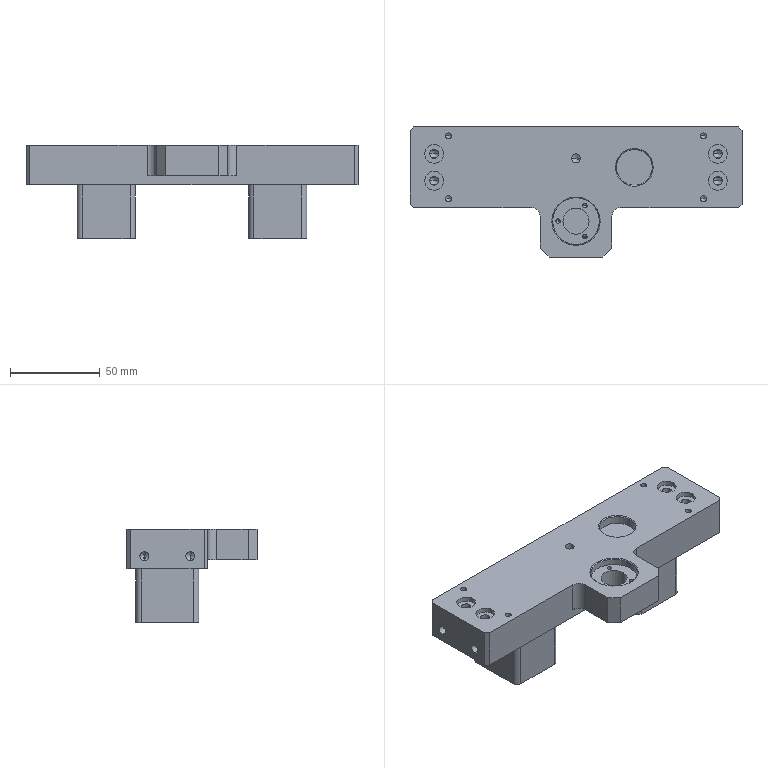NC program | NX | posted with a generic post | part box 185 x 72.5 x 52 mm
Whole program:
N10 G17 G21 G94 G90
(ZLEVEL_PROFILE_1 , TOOL : D10)
N12 T15 M6
N14 G54
N16 G17 G0 G90 X-108.145 Y0.067 S9500 M3
N18 G43 Z30. H15
N20 Z3.429
N22 G94 G1 Z2.429 F1000.
N24 X-107.651 Y0.199
N26 G2 X-106.685 Y-0.06 R1.
N28 G1 X-96.649 Y-10.096 F2500.
N30 X-96.62 Y-10.084
N32 G3 X-96.248 Y-10.498 R5.3
N34 G1 X-94.248 Y-12.498
N36 G3 X-90.5 Y-14.05 R5.3
N38 G1 X-25.3
N40 Y-30.19
N42 X-25.296 Y-30.622
N44 X-25.269 Y-30.673
N46 G3 X-23.748 Y-34.998 R5.3
N48 G1 X-18.748 Y-39.998
N50 G3 X-15. Y-41.55 R5.3
N52 G1 X15.
N54 G3 X18.748 Y-39.998 R5.3
N56 G1 X23.748 Y-34.998
N58 G3 X25.269 Y-30.673 R5.3
N60 G1 X25.296 Y-30.622
N62 Y-30.238
N64 X25.3 Y-30.19
N66 Y-14.05
N68 X90.5
N70 G3 X94.763 Y-11.9 R5.3
N72 G1 X94.829 Y-11.911
N74 X94.952 Y-11.788
N76 X94.979 Y-11.766
N78 X96.218 Y-10.527
N80 X106.852 Y0.107
N82 G2 X107.818 Y0.366 R1.
N84 G1 X108.268 Y0.246
N86 Z3.429
N88 G0 Z68.
N90 X-108.145 Y0.067
N92 Z2.857
N94 G1 Z1.857 F1000.
N96 X-107.651 Y0.199
N98 G2 X-106.685 Y-0.06 R1.
N100 G1 X-96.649 Y-10.096 F2500.
N102 X-96.62 Y-10.084
N104 G3 X-96.248 Y-10.498 R5.3
N106 G1 X-94.248 Y-12.498
N108 G3 X-90.5 Y-14.05 R5.3
N110 G1 X-25.3
N112 Y-30.19
N114 X-25.296 Y-30.622
N116 X-25.269 Y-30.673
N118 G3 X-23.748 Y-34.998 R5.3
N120 G1 X-18.748 Y-39.998
N122 G3 X-15. Y-41.55 R5.3
N124 G1 X15.
N126 G3 X18.748 Y-39.998 R5.3
N128 G1 X23.748 Y-34.998
N130 G3 X25.269 Y-30.673 R5.3
N132 G1 X25.296 Y-30.622
N134 Y-30.238
N136 X25.3 Y-30.19
N138 Y-14.05
N140 X90.5
N142 G3 X94.763 Y-11.9 R5.3
N144 G1 X94.829 Y-11.911
N146 X94.952 Y-11.788
N148 X94.979 Y-11.766
N150 X96.218 Y-10.527
N152 X106.852 Y0.107
N154 G2 X107.818 Y0.366 R1.
N156 G1 X108.268 Y0.246
N158 Z2.857
N160 G0 Z68.
N162 X-108.145 Y0.067
N164 Z2.286
N166 G1 Z1.286 F1000.
N168 X-107.651 Y0.199
N170 G2 X-106.685 Y-0.06 R1.
N172 G1 X-96.649 Y-10.096 F2500.
N174 X-96.62 Y-10.084
N176 G3 X-96.248 Y-10.498 R5.3
N178 G1 X-94.248 Y-12.498
N180 G3 X-90.5 Y-14.05 R5.3
N182 G1 X-25.3
N184 Y-30.19
N186 X-25.296 Y-30.622
N188 X-25.269 Y-30.673
N190 G3 X-23.748 Y-34.998 R5.3
N192 G1 X-18.748 Y-39.998
N194 G3 X-15. Y-41.55 R5.3
N196 G1 X15.
N198 G3 X18.748 Y-39.998 R5.3
N200 G1 X23.748 Y-34.998
N202 G3 X25.269 Y-30.673 R5.3
N204 G1 X25.296 Y-30.622
N206 Y-30.238
N208 X25.3 Y-30.19
N210 Y-14.05
N212 X90.5
N214 G3 X94.763 Y-11.9 R5.3
N216 G1 X94.829 Y-11.911
N218 X94.952 Y-11.788
N220 X94.979 Y-11.766
N222 X96.218 Y-10.527
N224 X106.852 Y0.107
N226 G2 X107.818 Y0.366 R1.
N228 G1 X108.268 Y0.246
N230 Z2.286
N232 G0 Z68.
N234 X-108.145 Y0.067
N236 Z1.714
N238 G1 Z0.714 F1000.
N240 X-107.651 Y0.199
N242 G2 X-106.685 Y-0.06 R1.
N244 G1 X-96.649 Y-10.096 F2500.
N246 X-96.62 Y-10.084
N248 G3 X-96.248 Y-10.498 R5.3
N250 G1 X-94.248 Y-12.498
N252 G3 X-90.5 Y-14.05 R5.3
N254 G1 X-25.3
N256 Y-30.19
N258 X-25.296 Y-30.622
N260 X-25.269 Y-30.673
N262 G3 X-23.748 Y-34.998 R5.3
N264 G1 X-18.748 Y-39.998
N266 G3 X-15. Y-41.55 R5.3
N268 G1 X15.
N270 G3 X18.748 Y-39.998 R5.3
N272 G1 X23.748 Y-34.998
N274 G3 X25.269 Y-30.673 R5.3
N276 G1 X25.296 Y-30.622
N278 Y-30.238
N280 X25.3 Y-30.19
N282 Y-14.05
N284 X90.5
N286 G3 X94.763 Y-11.9 R5.3
N288 G1 X94.829 Y-11.911
N290 X94.952 Y-11.788
N292 X94.979 Y-11.766
N294 X96.218 Y-10.527
N296 X106.852 Y0.107
N298 G2 X107.818 Y0.366 R1.
N300 G1 X108.268 Y0.246
N302 Z1.714
N304 G0 Z68.
N306 X-108.145 Y0.067
N308 Z1.143
N310 G1 Z0.143 F1000.
N312 X-107.651 Y0.199
N314 G2 X-106.685 Y-0.06 R1.
N316 G1 X-96.649 Y-10.096 F2500.
N318 X-96.62 Y-10.084
N320 G3 X-96.248 Y-10.498 R5.3
N322 G1 X-94.248 Y-12.498
N324 G3 X-90.5 Y-14.05 R5.3
N326 G1 X-25.3
N328 Y-30.19
N330 X-25.296 Y-30.622
N332 X-25.269 Y-30.673
N334 G3 X-23.748 Y-34.998 R5.3
N336 G1 X-18.748 Y-39.998
N338 G3 X-15. Y-41.55 R5.3
N340 G1 X15.
N342 G3 X18.748 Y-39.998 R5.3
N344 G1 X23.748 Y-34.998
N346 G3 X25.269 Y-30.673 R5.3
N348 G1 X25.296 Y-30.622
N350 Y-30.238
N352 X25.3 Y-30.19
N354 Y-14.05
N356 X90.5
N358 G3 X94.763 Y-11.9 R5.3
N360 G1 X94.829 Y-11.911
N362 X94.952 Y-11.788
N364 X94.979 Y-11.766
N366 X96.218 Y-10.527
N368 X106.852 Y0.107
N370 G2 X107.818 Y0.366 R1.
N372 G1 X108.268 Y0.246
N374 Z1.143
N376 G0 Z68.
N378 X-108.145 Y0.067
N380 Z0.571
N382 G1 Z-0.429 F1000.
N384 X-107.651 Y0.199
N386 G2 X-106.685 Y-0.06 R1.
N388 G1 X-96.649 Y-10.096 F2500.
N390 X-96.62 Y-10.084
N392 G3 X-96.248 Y-10.498 R5.3
N394 G1 X-94.248 Y-12.498
N396 G3 X-90.5 Y-14.05 R5.3
N398 G1 X-25.3
N400 Y-30.19
N402 X-25.296 Y-30.622
N404 X-25.269 Y-30.673
N406 G3 X-23.748 Y-34.998 R5.3
N408 G1 X-18.748 Y-39.998
N410 G3 X-15. Y-41.55 R5.3
N412 G1 X15.
N414 G3 X18.748 Y-39.998 R5.3
N416 G1 X23.748 Y-34.998
N418 G3 X25.269 Y-30.673 R5.3
N420 G1 X25.296 Y-30.622
N422 Y-30.238
N424 X25.3 Y-30.19
N426 Y-14.05
N428 X90.5
N430 G3 X94.763 Y-11.9 R5.3
N432 G1 X94.829 Y-11.911
N434 X94.952 Y-11.788
N436 X94.979 Y-11.766
N438 X96.218 Y-10.527
N440 X106.852 Y0.107
N442 G2 X107.818 Y0.366 R1.
N444 G1 X108.268 Y0.246
N446 Z0.571
N448 G0 Z68.
N450 X-108.145 Y0.067
N452 Z0.
N454 G1 Z-1. F1000.
N456 X-107.651 Y0.199
N458 G2 X-106.685 Y-0.06 R1.
N460 G1 X-96.649 Y-10.096 F2500.
N462 X-96.62 Y-10.084
N464 G3 X-96.248 Y-10.498 R5.3
N466 G1 X-94.248 Y-12.498
N468 G3 X-90.5 Y-14.05 R5.3
N470 G1 X-25.3
N472 Y-30.19
N474 X-25.296 Y-30.622
N476 X-25.269 Y-30.673
N478 G3 X-23.748 Y-34.998 R5.3
N480 G1 X-18.748 Y-39.998
N482 G3 X-15. Y-41.55 R5.3
N484 G1 X15.
N486 G3 X18.748 Y-39.998 R5.3
N488 G1 X23.748 Y-34.998
N490 G3 X25.269 Y-30.673 R5.3
N492 G1 X25.296 Y-30.622
N494 Y-30.238
N496 X25.3 Y-30.19
N498 Y-14.05
N500 X90.5
N502 G3 X94.763 Y-11.9 R5.3
N504 G1 X94.829 Y-11.911
N506 X94.952 Y-11.788
N508 X94.979 Y-11.766
N510 X96.218 Y-10.527
N512 X106.852 Y0.107
N514 G2 X107.818 Y0.366 R1.
N516 G1 X108.268 Y0.246
N518 Z0.
N520 G0 Z30.
N522 M5
(FLOOR_WALL_COPY_COPY , TOOL : D80)
N524 T19 M6
N526 G54
N528 G17 G0 G90 X-137.5 Y36.247 S6500 M3
N530 G43 Z30. H19
N532 Z5.
N534 G94 G1 Z2. F1500.
N536 X-132.5
N538 X132.5
N540 Y-4.25
N542 X-132.5
N544 X-137.5
N546 Z5.
N548 G0 Z30.
N550 Y36.247
N552 Z4.
N554 G1 Z1.
N556 X-132.5
N558 X132.5
N560 Y-4.25
N562 X-132.5
N564 X-137.5
N566 Z4.
N568 G0 Z30.
N570 Y36.247
N572 Z3.
N574 G1 Z0.
N576 X-132.5
N578 X132.5
N580 Y-4.25
N582 X-132.5
N584 X-137.5
N586 Z3.
N588 G0 Z30.
N590 M5
(DRILLING_COPY_1_COPY , TOOL : D6A45)
N592 T01 M6
N594 G54
N596 G17 G0 G90 X71. Y-3.75 S5000 M3
N598 G43 Z30. H1
N600 G94 G81 G98 Z-1. F350. R3.
N602 X79. Y6.25
N604 Y21.25
N606 X71. Y31.25
N608 X32.5 Y13.75
N610 X0. Y18.75
N612 X5. Y-7.59
N614 X0. Y-16.25
N616 X5. Y-24.91
N618 X-10. Y-16.25
N620 X-71. Y-3.75
N622 X-79. Y6.25
N624 Y21.25
N626 X-71. Y31.25
N628 G80
N630 G0 X-71. Y31.25 Z30.
N632 M5
(DRILLING_COPY_COPY_1 , TOOL : 3.3ZT)
N634 T03 M6
N636 G54
N638 G17 G0 G90 X-71. Y-3.75 S2000 M3
N640 G43 Z30. H3
N642 G94 G83 G98 Z-10.491 F180. Q2. R3.
N644 Y31.25
N646 X71.
N648 Y-3.75
N650 G80
N652 G0 X71. Y-3.75 Z30.
(DRILLING_COPY_COPY_1_COPY_1 , TOOL : 3.3ZT)
N654 X0. Y18.75
N656 G83 Z-8.491 F180. Q2. R3.
N658 G80
N660 G0 X0. Y18.75 Z30.
N662 M5
(DRILLING_COPY_COPY_1_COPY , TOOL : 2.5ZT)
N664 T02 M6
N666 G54
N668 G17 G0 G90 X-10. Y-16.25 S2006 M3
N670 G43 Z30. H2
N672 G94 G83 G98 Z-12.251 F120. Q2. R3.
N674 X5. Y-24.91
N676 Y-7.59
N678 G80
N680 G0 X5. Y-7.59 Z30.
N682 M5
(DRILLING_COPY_COPY_COPY , TOOL : 5.0ZT)
N684 T05 M6
N686 G54
N688 G17 G0 G90 X-79. Y21.25 S1516 M3
N690 G43 Z30. H5
N692 G94 G83 G98 Z-18.002 F180. Q2. R3.
N694 Y6.25
N696 X79.
N698 Y21.25
N700 G80
N702 G0 X79. Y21.25 Z30.
N704 M5
(HOLE_MILLING , TOOL : D10)
N706 T15 M6
N708 G54
N710 G17 G0 G90 X0. Y-16.25 S9500 M3
N712 G43 Z30. H15
N714 Z1.
N716 G94 G3 X1.975 Y-18.225 R1.975 F2200.
N718 X3.95 Y-16.25 R1.975
N720 X3.95 Y-16.25 Z0. I-3.95 J0.
N722 X3.95 Y-16.25 Z-1. I-3.95 J0.
N724 X3.95 Y-16.25 Z-2. I-3.95 J0.
N726 X3.95 Y-16.25 Z-3. I-3.95 J0.
N728 X3.95 Y-16.25 Z-4. I-3.95 J0.
N730 X3.757 Y-15.029 Z-4.05 R3.95
N732 X-1.221 Y-12.493 R3.95
N734 X3.757 Y-15.029 R-3.95
N736 X1.268 Y-13.761 R1.975
N738 X0. Y-16.25 R1.975
N740 G0 Z1.
N742 G3 X3.95 Y-20.2 R3.95
N744 X7.9 Y-16.25 R3.95
N746 X7.9 Y-16.25 Z0. I-7.9 J0.
N748 X7.9 Y-16.25 Z-1. I-7.9 J0.
N750 X7.9 Y-16.25 Z-2. I-7.9 J0.
N752 X7.9 Y-16.25 Z-3. I-7.9 J0.
N754 X7.9 Y-16.25 Z-4. I-7.9 J0.
N756 X7.513 Y-13.809 Z-4.05 R7.9
N758 X-2.441 Y-8.737 R7.9
N760 X7.513 Y-13.809 R-7.9
N762 X2.536 Y-11.273 R3.95
N764 X0. Y-16.25 R3.95
N766 G0 Z30.
N768 X32.5 Y13.75
N770 Z1.
N772 G3 X34.95 Y11.3 R2.45
N774 X37.4 Y13.75 R2.45
N776 X37.4 Y13.75 Z0. I-4.9 J0.
N778 X37.4 Y13.75 Z-1. I-4.9 J0.
N780 X37.4 Y13.75 Z-2. I-4.9 J0.
N782 X37.4 Y13.75 Z-3. I-4.9 J0.
N784 X37.4 Y13.75 Z-4. I-4.9 J0.
N786 X37.4 Y13.75 Z-5. I-4.9 J0.
N788 X32.5 Y18.65 R4.9
N790 X37.4 Y13.75 R-4.9
N792 X34.95 Y16.2 R2.45
N794 X32.5 Y13.75 R2.45
N796 G0 Z30.
(HOLE_MILLING_COPY , TOOL : D10)
N798 X0. Y-16.25
N800 Z-3.05
N802 G3 X1.075 Y-17.325 R1.075
N804 X2.15 Y-16.25 R1.075
N806 X2.15 Y-16.25 Z-4.05 I-2.15 J0.
N808 X2.15 Y-16.25 Z-5.05 I-2.15 J0.
N810 X2.15 Y-16.25 Z-6.05 I-2.15 J0.
N812 X2.15 Y-16.25 Z-7.05 I-2.15 J0.
N814 X2.15 Y-16.25 Z-8.05 I-2.15 J0.
N816 X2.15 Y-16.25 Z-9.05 I-2.15 J0.
N818 X2.15 Y-16.25 Z-10.05 I-2.15 J0.
N820 X2.15 Y-16.25 Z-11.05 I-2.15 J0.
N822 X2.15 Y-16.25 Z-12.05 I-2.15 J0.
N824 X2.15 Y-16.25 Z-13.05 I-2.15 J0.
N826 X2.15 Y-16.25 Z-14.05 I-2.15 J0.
N828 X2.045 Y-16.914 Z-15. R-2.15
N830 X0.664 Y-14.205 R2.15
N832 X2.045 Y-16.914 R-2.15
N834 X1.355 Y-15.56 R1.075
N836 X0. Y-16.25 R1.075
N838 G0 Z30.
N840 M5
(HOLE_MILLING_COPY_COPY , TOOL : D6)
N842 T12 M6
N844 G54
N846 G17 G0 G90 X-79. Y21.25 S9500 M3
N848 G43 Z30. H12
N850 Z1.
N852 G94 G3 X-77.875 Y20.125 R1.125 F1650.
N854 X-76.75 Y21.25 R1.125
N856 X-76.75 Y21.25 Z0.5 I-2.25 J0.
N858 X-76.75 Y21.25 Z0. I-2.25 J0.
N860 X-76.75 Y21.25 Z-0.5 I-2.25 J0.
N862 X-76.75 Y21.25 Z-1. I-2.25 J0.
N864 X-76.75 Y21.25 Z-1.5 I-2.25 J0.
N866 X-76.75 Y21.25 Z-2. I-2.25 J0.
N868 X-76.75 Y21.25 Z-2.5 I-2.25 J0.
N870 X-80.82 Y22.573 Z-2.7 R2.25
N872 X-80.323 Y19.43 R2.25
N874 X-80.82 Y22.573 R-2.25
N876 X-80.571 Y21.001 R1.125
N878 X-79. Y21.25 R1.125
N880 G0 Z30.
N882 Y6.25
N884 Z1.
N886 G3 X-77.875 Y5.125 R1.125
N888 X-76.75 Y6.25 R1.125
N890 X-76.75 Y6.25 Z0.5 I-2.25 J0.
N892 X-76.75 Y6.25 Z0. I-2.25 J0.
N894 X-76.75 Y6.25 Z-0.5 I-2.25 J0.
N896 X-76.75 Y6.25 Z-1. I-2.25 J0.
N898 X-76.75 Y6.25 Z-1.5 I-2.25 J0.
N900 X-76.75 Y6.25 Z-2. I-2.25 J0.
N902 X-76.75 Y6.25 Z-2.5 I-2.25 J0.
N904 X-80.82 Y7.573 Z-2.7 R2.25
N906 X-80.323 Y4.43 R2.25
N908 X-80.82 Y7.573 R-2.25
N910 X-80.571 Y6.001 R1.125
N912 X-79. Y6.25 R1.125
N914 G0 Z30.
N916 X79.
N918 Z1.
N920 G3 X80.125 Y5.125 R1.125
N922 X81.25 Y6.25 R1.125
N924 X81.25 Y6.25 Z0.5 I-2.25 J0.
N926 X81.25 Y6.25 Z0. I-2.25 J0.
N928 X81.25 Y6.25 Z-0.5 I-2.25 J0.
N930 X81.25 Y6.25 Z-1. I-2.25 J0.
N932 X81.25 Y6.25 Z-1.5 I-2.25 J0.
N934 X81.25 Y6.25 Z-2. I-2.25 J0.
N936 X81.25 Y6.25 Z-2.5 I-2.25 J0.
N938 X77.18 Y7.573 Z-2.7 R2.25
N940 X77.677 Y4.43 R2.25
N942 X77.18 Y7.573 R-2.25
N944 X77.429 Y6.001 R1.125
N946 X79. Y6.25 R1.125
N948 G0 Z30.
N950 Y21.25
N952 Z1.
N954 G3 X80.125 Y20.125 R1.125
N956 X81.25 Y21.25 R1.125
N958 X81.25 Y21.25 Z0.5 I-2.25 J0.
N960 X81.25 Y21.25 Z0. I-2.25 J0.
N962 X81.25 Y21.25 Z-0.5 I-2.25 J0.
N964 X81.25 Y21.25 Z-1. I-2.25 J0.
N966 X81.25 Y21.25 Z-1.5 I-2.25 J0.
N968 X81.25 Y21.25 Z-2. I-2.25 J0.
N970 X81.25 Y21.25 Z-2.5 I-2.25 J0.
N972 X77.18 Y22.573 Z-2.7 R2.25
N974 X77.677 Y19.43 R2.25
N976 X77.18 Y22.573 R-2.25
N978 X77.429 Y21.001 R1.125
N980 X79. Y21.25 R1.125
N982 G0 Z30.
N984 M5
(HOLE_MILLING_COPY_COPY_COPY , TOOL : D3)
N986 T17 M6
N988 G54
N990 G17 G0 G90 X0. Y18.75 S9500 M3
N992 G43 Z30. H17
N994 Z1.
N996 G94 G3 X0.45 Y18.3 R0.45 F1200.
N998 X0.9 Y18.75 R0.45
N1000 X0.9 Y18.75 Z0.8 I-0.9 J0.
N1002 X0.9 Y18.75 Z0.6 I-0.9 J0.
N1004 X0.9 Y18.75 Z0.4 I-0.9 J0.
N1006 X0.9 Y18.75 Z0.2 I-0.9 J0.
N1008 X0.9 Y18.75 Z0. I-0.9 J0.
N1010 X0.9 Y18.75 Z-0.2 I-0.9 J0.
N1012 X0.9 Y18.75 Z-0.4 I-0.9 J0.
N1014 X0.9 Y18.75 Z-0.6 I-0.9 J0.
N1016 X0.9 Y18.75 Z-0.8 I-0.9 J0.
N1018 X0.9 Y18.75 Z-1. I-0.9 J0.
N1020 X0.9 Y18.75 Z-1.2 I-0.9 J0.
N1022 X0.9 Y18.75 Z-1.4 I-0.9 J0.
N1024 X0.9 Y18.75 Z-1.6 I-0.9 J0.
N1026 X0.9 Y18.75 Z-1.8 I-0.9 J0.
N1028 X0.9 Y18.75 Z-2. I-0.9 J0.
N1030 X0.9 Y18.75 Z-2.2 I-0.9 J0.
N1032 X0.9 Y18.75 Z-2.4 I-0.9 J0.
N1034 X0.9 Y18.75 Z-2.6 I-0.9 J0.
N1036 X0.9 Y18.75 Z-2.8 I-0.9 J0.
N1038 X0.9 Y18.75 Z-3. I-0.9 J0.
N1040 X0.9 Y18.75 Z-3.2 I-0.9 J0.
N1042 X0.9 Y18.75 Z-3.4 I-0.9 J0.
N1044 X0.9 Y18.75 Z-3.6 I-0.9 J0.
N1046 X0.9 Y18.75 Z-3.8 I-0.9 J0.
N1048 X0.9 Y18.75 Z-4. I-0.9 J0.
N1050 X0.9 Y18.75 Z-4.2 I-0.9 J0.
N1052 X0.9 Y18.75 Z-4.4 I-0.9 J0.
N1054 X0.9 Y18.75 Z-4.6 I-0.9 J0.
N1056 X0.9 Y18.75 Z-4.8 I-0.9 J0.
N1058 X0.9 Y18.75 Z-5. I-0.9 J0.
N1060 X0.9 Y18.75 Z-5.2 I-0.9 J0.
N1062 X0.9 Y18.75 Z-5.4 I-0.9 J0.
N1064 X0.9 Y18.75 Z-5.6 I-0.9 J0.
N1066 X0.9 Y18.75 Z-5.8 I-0.9 J0.
N1068 X0.9 Y18.75 Z-6. I-0.9 J0.
N1070 X0.9 Y18.75 Z-6.2 I-0.9 J0.
N1072 X0.9 Y18.75 Z-6.4 I-0.9 J0.
N1074 X0.9 Y18.75 Z-6.6 I-0.9 J0.
N1076 X0.9 Y18.75 Z-6.8 I-0.9 J0.
N1078 X0.9 Y18.75 Z-7. I-0.9 J0.
N1080 X0.9 Y18.75 Z-7.2 I-0.9 J0.
N1082 X0.9 Y18.75 Z-7.4 I-0.9 J0.
N1084 X-0.9 Y18.75 Z-7.5 I-0.9 J0.
N1086 X0. Y17.85 R0.9
N1088 X-0.9 Y18.75 R-0.9
N1090 X-0.45 Y18.3 R0.45
N1092 X0. Y18.75 R0.45
N1094 G0 Z30.
N1096 M5
(FLOOR_WALL_COPY_1 , TOOL : D10JING)
N1098 T14 M6
N1100 G54
N1102 G17 G0 G90 X33.495 Y13.847 S9500 M3
N1104 G43 Z30. H14
N1106 Z-3.5
N1108 G94 G1 Z-5. F1250.
N1110 G3 X32.5 Y13.75 R1.
N1112 G1 X37.
N1114 G3 X32.5 Y18.25 R4.5
N1116 X37. Y13.75 R-4.5
N1118 G1 Y12.884
N1120 G3 X37.5 Y13.75 R1.
N1122 X32.5 Y18.75 R5.
N1124 X37.5 Y13.75 R-5.
N1126 X37. Y14.616 R1.
N1128 G1 X35.561 Y15.447
N1130 Z-3.5
N1132 G0 Z30.
N1134 X-0.866 Y-17.5
N1136 Z-13.5
N1138 G1 Z-15.
N1140 G3 X0. Y-18. R1.
N1142 X1.75 Y-16.25 R1.75
N1144 X0. Y-18. R-1.75
N1146 G1 X-0.866
N1148 G3 X0. Y-18.5 R1.
N1150 X2.25 Y-16.25 R2.25
N1152 X0. Y-18.5 R-2.25
N1154 X0.866 Y-18. R1.
N1156 G1 X0.333 Y-16.922
N1158 Z-13.5
N1160 G0 Z30.
N1162 M5
(PLANAR_MILL_COPY_COPY_COPY_COPY_COPY_COPY_1_COPY_1 , TOOL : D6A45)
N1164 T01 M6
N1166 G54
N1168 G17 G0 G90 X-70.567 Y31.75 S9500 M3
N1170 G43 Z30. H1
N1172 Z0.5
N1174 G94 G1 Z-1. F1250.
N1176 G3 X-71. Y32. R0.5
N1178 X-71.75 Y31.25 R0.75
N1180 X-71. Y32. R-0.75
N1182 X-71.433 Y31.75 R0.5
N1184 G1 Z0.5
N1186 G0 Z30.
N1188 X-78.134 Y25.1
N1190 Z0.5
N1192 G1 Z-1.
N1194 G3 X-79. Y25.6 R1.
N1196 X-83.35 Y21.25 R4.35
N1198 X-79. Y25.6 R-4.35
N1200 X-79.866 Y25.1 R1.
N1202 G1 Z0.5
N1204 G0 Z30.
N1206 X-82.85 Y7.116
N1208 Z0.5
N1210 G1 Z-1.
N1212 G3 X-83.35 Y6.25 R1.
N1214 X-79. Y1.9 R4.35
N1216 X-83.35 Y6.25 R-4.35
N1218 X-82.85 Y5.384 R1.
N1220 G1 Z0.5
N1222 G0 Z30.
N1224 X-71.5 Y-3.317
N1226 Z0.5
N1228 G1 Z-1.
N1230 G3 X-71.75 Y-3.75 R0.5
N1232 X-71. Y-4.5 R0.75
N1234 X-71.75 Y-3.75 R-0.75
N1236 X-71.5 Y-4.183 R0.5
N1238 G1 Z0.5
N1240 G0 Z30.
N1242 X-0.866 Y37.65
N1244 Z0.5
N1246 G1 Z-1.
N1248 G3 X0. Y37.15 R1.
N1250 G1 X90.5
N1252 G2 X91.136 Y36.886 R0.9
N1254 G1 X93.136 Y34.886
N1256 G2 X93.4 Y34.25 R0.9
N1258 G1 Y-6.75
N1260 G2 X93.136 Y-7.386 R0.9
N1262 G1 X91.136 Y-9.386
N1264 G2 X90.5 Y-9.65 R0.9
N1266 G1 X25.
N1268 G3 X20.9 Y-13.75 R4.1
N1270 G1 Y-31.25
N1272 G2 X20.636 Y-31.886 R0.9
N1274 G1 X15.636 Y-36.886
N1276 G2 X15. Y-37.15 R0.9
N1278 G1 X-15.
N1280 G2 X-15.636 Y-36.886 R0.9
N1282 G1 X-20.636 Y-31.886
N1284 G2 X-20.9 Y-31.25 R0.9
N1286 G1 Y-13.75
N1288 G3 X-25. Y-9.65 R4.1
N1290 G1 X-90.5
N1292 G2 X-91.136 Y-9.386 R0.9
N1294 G1 X-93.136 Y-7.386
N1296 G2 X-93.4 Y-6.75 R0.9
N1298 G1 Y34.25
N1300 G2 X-93.136 Y34.886 R0.9
N1302 G1 X-91.136 Y36.886
N1304 G2 X-90.5 Y37.15 R0.9
N1306 G1 X0.
N1308 G3 X0.866 Y37.65 R1.
N1310 G1 Z0.5
N1312 G0 Z30.
N1314 Y19.85
N1316 Z0.5
N1318 G1 Z-1.
N1320 G3 X0. Y20.35 R1.
N1322 X-1.6 Y18.75 R1.6
N1324 X0. Y20.35 R-1.6
N1326 X-0.866 Y19.85 R1.
N1328 G1 Z0.5
N1330 G0 Z30.
N1332 X71.433 Y31.75
N1334 Z0.5
N1336 G1 Z-1.
N1338 G3 X71. Y32. R0.5
N1340 X70.25 Y31.25 R0.75
N1342 X71. Y32. R-0.75
N1344 X70.567 Y31.75 R0.5
N1346 G1 Z0.5
N1348 G0 Z30.
N1350 X79.866 Y25.1
N1352 Z0.5
N1354 G1 Z-1.
N1356 G3 X79. Y25.6 R1.
N1358 X74.65 Y21.25 R4.35
N1360 X79. Y25.6 R-4.35
N1362 X78.134 Y25.1 R1.
N1364 G1 Z0.5
N1366 G0 Z30.
N1368 X82.85 Y5.384
N1370 Z0.5
N1372 G1 Z-1.
N1374 G3 X83.35 Y6.25 R1.
N1376 X79. Y10.6 R4.35
N1378 X83.35 Y6.25 R-4.35
N1380 X82.85 Y7.116 R1.
N1382 G1 Z0.5
N1384 G0 Z30.
N1386 X71.5 Y-4.183
N1388 Z0.5
N1390 G1 Z-1.
N1392 G3 X71.75 Y-3.75 R0.5
N1394 X71. Y-3. R0.75
N1396 X71.75 Y-3.75 R-0.75
N1398 X71.5 Y-3.317 R0.5
N1400 G1 Z0.5
N1402 G0 Z30.
(PLANAR_MILL_COPY_COPY_COPY_COPY_COPY_COPY_1_COPY_1_COPY , TOOL : D6A45)
N1404 X12. Y-17.116
N1406 Z0.5
N1408 G1 Z-1.
N1410 G3 X12.5 Y-16.25 R1.
N1412 X0. Y-3.75 R12.5
N1414 X12.5 Y-16.25 R-12.5
N1416 X12. Y-15.384 R1.
N1418 G1 Z0.5
N1420 G0 Z30.
N1422 X41.5 Y12.884
N1424 Z0.5
N1426 G1 Z-1.
N1428 G3 X42. Y13.75 R1.
N1430 X32.5 Y23.25 R9.5
N1432 X42. Y13.75 R-9.5
N1434 X41.5 Y14.616 R1.
N1436 G1 Z0.5
N1438 G0 Z30.
N1440 M5
(刀补 , TOOL : D10JING)
N1442 T14 M6
N1444 G54
N1446 G17 G0 G90 X-1.895 Y-21.571 S9500 M3
N1448 G43 Z30. H14
N1450 Z-2.55
N1452 G94 G1 Z-4.05 F1250.
N1454 G41 X-1.553 Y-22.51 D14
N1456 X-0.866 Y-23.7
N1458 G3 X0. Y-24.2 R1.
N1460 X7.95 Y-16.25 R7.95
N1462 X0. Y-24.2 R-7.95
N1464 X0.866 Y-23.7 R1.
N1466 G1 X1.553 Y-22.51
N1468 G40
N1470 X1.895 Y-21.571
N1472 Z-2.55
N1474 G0 Z30.
N1476 M5
(刀补17 , TOOL : D3)
N1478 T17 M6
N1480 G54
N1482 G17 G0 G90 X0. Y18.75 S9500 M3
N1484 G43 Z30. H17
N1486 Z1.
N1488 G41 G94 G1 X0.004 Y18.65 F850. D17
N1490 G3 X0.95 Y18.75 R0.478
N1492 X0.95 Y18.75 Z-1. I-0.95 J0.
N1494 X0.95 Y18.75 Z-3. I-0.95 J0.
N1496 X0.95 Y18.75 Z-5. I-0.95 J0.
N1498 X0.95 Y18.75 Z-7. I-0.95 J0.
N1500 X0. Y19.7 Z-7.5 R0.95
N1502 X-0.95 Y18.75 R0.95
N1504 X0. Y19.7 R-0.95
N1506 X-0.1 Y18.754 R0.478
N1508 G40
N1510 G1 X0. Y18.75
N1512 G0 Z30.
N1514 M5
N1516 M2